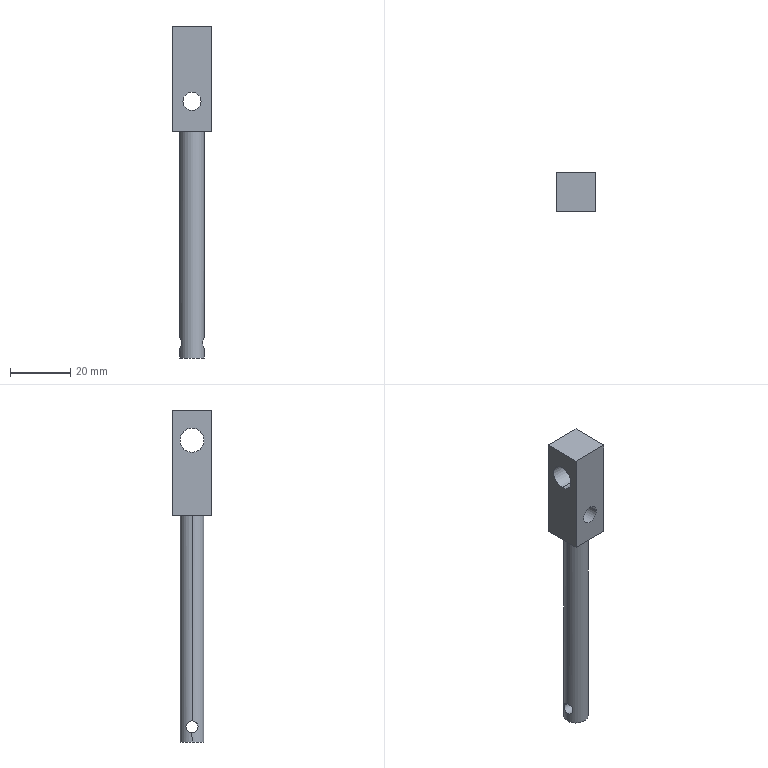Part | SolidWorks | features ICE 5, Extrusion 1 | 1 solid | 15 faces | box 13 x 13 x 110 mm | volume 8567 mm3 | cylinder 8 | plane 7 | commonest cylinder face diameters 8 x4 4 x2 6 x2
STEP:
#1=CARTESIAN_POINT('',(3.464,2.,-80.));
#2=VERTEX_POINT('',#1);
#3=CARTESIAN_POINT('',(4.,0.,-82.));
#4=VERTEX_POINT('',#3);
#5=CARTESIAN_POINT('',(3.464,2.,-80.));
#6=CARTESIAN_POINT('',(3.464,2.,-80.132));
#7=CARTESIAN_POINT('',(3.472,1.987,-80.266));
#8=CARTESIAN_POINT('',(3.501,1.934,-80.526));
#9=CARTESIAN_POINT('',(3.523,1.895,-80.652));
#10=CARTESIAN_POINT('',(3.602,1.744,-81.014));
#11=CARTESIAN_POINT('',(3.673,1.597,-81.231));
#12=CARTESIAN_POINT('',(3.776,1.324,-81.505));
#13=CARTESIAN_POINT('',(3.81,1.225,-81.586));
#14=CARTESIAN_POINT('',(3.872,1.011,-81.731));
#15=CARTESIAN_POINT('',(3.901,0.8943,-81.794));
#16=CARTESIAN_POINT('',(3.948,0.6536,-81.895));
#17=CARTESIAN_POINT('',(3.967,0.5287,-81.933));
#18=CARTESIAN_POINT('',(3.993,0.2692,-81.986));
#19=CARTESIAN_POINT('',(4.,0.1343,-82.));
#20=CARTESIAN_POINT('',(4.,0.,-82.));
#21=B_SPLINE_CURVE_WITH_KNOTS('',3,(#5,#6,#7,#8,#9,#10,#11,#12,#13,#14,#15,#16,#17,#18,#19,#20),.UNSPECIFIED.,.F.,.F.,(4,2,2,2,2,2,2,4),(0.00954,0.009936,0.01033,0.01113,0.01152,0.01192,0.01232,0.01271),.UNSPECIFIED.);
#22=EDGE_CURVE('',#2,#4,#21,.T.);
#23=ORIENTED_EDGE('',*,*,#22,.F.);
#24=CARTESIAN_POINT('',(-3.464,2.,-80.));
#25=VERTEX_POINT('',#24);
#26=CARTESIAN_POINT('',(293.5,2.,-80.));
#27=DIRECTION('',(-1.,0.,0.));
#28=VECTOR('',#27,1000.);
#29=LINE('',#26,#28);
#30=EDGE_CURVE('',#2,#25,#29,.T.);
#31=ORIENTED_EDGE('',*,*,#30,.T.);
#32=CARTESIAN_POINT('',(-4.,0.,-82.));
#33=VERTEX_POINT('',#32);
#34=CARTESIAN_POINT('',(-4.,0.,-82.));
#35=CARTESIAN_POINT('',(-4.,0.1332,-82.));
#36=CARTESIAN_POINT('',(-3.993,0.2678,-81.986));
#37=CARTESIAN_POINT('',(-3.967,0.5267,-81.934));
#38=CARTESIAN_POINT('',(-3.948,0.6539,-81.895));
#39=CARTESIAN_POINT('',(-3.9,0.8967,-81.793));
#40=CARTESIAN_POINT('',(-3.872,1.011,-81.731));
#41=CARTESIAN_POINT('',(-3.809,1.226,-81.586));
#42=CARTESIAN_POINT('',(-3.775,1.326,-81.502));
#43=CARTESIAN_POINT('',(-3.672,1.598,-81.23));
#44=CARTESIAN_POINT('',(-3.601,1.745,-81.011));
#45=CARTESIAN_POINT('',(-3.523,1.895,-80.652));
#46=CARTESIAN_POINT('',(-3.501,1.934,-80.525));
#47=CARTESIAN_POINT('',(-3.472,1.987,-80.264));
#48=CARTESIAN_POINT('',(-3.464,2.,-80.133));
#49=CARTESIAN_POINT('',(-3.464,2.,-80.));
#50=B_SPLINE_CURVE_WITH_KNOTS('',3,(#34,#35,#36,#37,#38,#39,#40,#41,#42,#43,#44,#45,#46,#47,#48,#49),.UNSPECIFIED.,.F.,.F.,(4,2,2,2,2,2,2,4),(0.003182,0.003579,0.003977,0.004374,0.004772,0.005566,0.005964,0.006361),.UNSPECIFIED.);
#51=EDGE_CURVE('',#33,#25,#50,.T.);
#52=ORIENTED_EDGE('',*,*,#51,.F.);
#53=CARTESIAN_POINT('',(-3.464,-2.,-80.));
#54=VERTEX_POINT('',#53);
#55=CARTESIAN_POINT('',(-3.464,-2.,-80.));
#56=CARTESIAN_POINT('',(-3.464,-2.,-80.135));
#57=CARTESIAN_POINT('',(-3.472,-1.987,-80.267));
#58=CARTESIAN_POINT('',(-3.501,-1.934,-80.525));
#59=CARTESIAN_POINT('',(-3.523,-1.895,-80.653));
#60=CARTESIAN_POINT('',(-3.602,-1.743,-81.015));
#61=CARTESIAN_POINT('',(-3.673,-1.596,-81.233));
#62=CARTESIAN_POINT('',(-3.81,-1.233,-81.596));
#63=CARTESIAN_POINT('',(-3.877,-1.014,-81.744));
#64=CARTESIAN_POINT('',(-3.948,-0.653,-81.895));
#65=CARTESIAN_POINT('',(-3.968,-0.5246,-81.935));
#66=CARTESIAN_POINT('',(-3.993,-0.2649,-81.987));
#67=CARTESIAN_POINT('',(-4.,-0.1333,-82.));
#68=CARTESIAN_POINT('',(-4.,0.,-82.));
#69=B_SPLINE_CURVE_WITH_KNOTS('',3,(#55,#56,#57,#58,#59,#60,#61,#62,#63,#64,#65,#66,#67,#68),.UNSPECIFIED.,.F.,.F.,(4,2,2,2,2,2,4),(0.,0.0003977,0.0007955,0.001591,0.002386,0.002784,0.003182),.UNSPECIFIED.);
#70=EDGE_CURVE('',#54,#33,#69,.T.);
#71=ORIENTED_EDGE('',*,*,#70,.F.);
#72=CARTESIAN_POINT('',(3.464,-2.,-80.));
#73=VERTEX_POINT('',#72);
#74=CARTESIAN_POINT('',(293.5,-2.,-80.));
#75=DIRECTION('',(-1.,0.,0.));
#76=VECTOR('',#75,1000.);
#77=LINE('',#74,#76);
#78=EDGE_CURVE('',#73,#54,#77,.T.);
#79=ORIENTED_EDGE('',*,*,#78,.F.);
#80=CARTESIAN_POINT('',(4.,0.,-82.));
#81=CARTESIAN_POINT('',(4.,-0.1347,-82.));
#82=CARTESIAN_POINT('',(3.993,-0.2667,-81.987));
#83=CARTESIAN_POINT('',(3.967,-0.5257,-81.934));
#84=CARTESIAN_POINT('',(3.948,-0.654,-81.895));
#85=CARTESIAN_POINT('',(3.877,-1.017,-81.742));
#86=CARTESIAN_POINT('',(3.809,-1.235,-81.594));
#87=CARTESIAN_POINT('',(3.672,-1.598,-81.23));
#88=CARTESIAN_POINT('',(3.601,-1.745,-81.012));
#89=CARTESIAN_POINT('',(3.523,-1.895,-80.652));
#90=CARTESIAN_POINT('',(3.501,-1.935,-80.524));
#91=CARTESIAN_POINT('',(3.472,-1.987,-80.265));
#92=CARTESIAN_POINT('',(3.464,-2.,-80.133));
#93=CARTESIAN_POINT('',(3.464,-2.,-80.));
#94=B_SPLINE_CURVE_WITH_KNOTS('',3,(#80,#81,#82,#83,#84,#85,#86,#87,#88,#89,#90,#91,#92,#93),.UNSPECIFIED.,.F.,.F.,(4,2,2,2,2,2,4),(0.,0.0003979,0.0007957,0.001591,0.002387,0.002785,0.003183),.UNSPECIFIED.);
#95=EDGE_CURVE('',#4,#73,#94,.T.);
#96=ORIENTED_EDGE('',*,*,#95,.F.);
#97=EDGE_LOOP('',(#23,#31,#52,#71,#79,#96));
#98=FACE_OUTER_BOUND('',#97,.T.);
#99=CARTESIAN_POINT('',(293.5,0.,-80.));
#100=DIRECTION('',(-1.,0.,0.));
#101=DIRECTION('',(0.,-1.,0.));
#102=AXIS2_PLACEMENT_3D('',#99,#100,#101);
#103=CYLINDRICAL_SURFACE('',#102,2.);
#104=ADVANCED_FACE('',(#98),#103,.F.);
#105=CARTESIAN_POINT('',(6.5,0.,11.));
#106=VERTEX_POINT('',#105);
#107=CARTESIAN_POINT('',(6.5,0.,19.));
#108=VERTEX_POINT('',#107);
#109=CARTESIAN_POINT('',(6.5,0.,15.));
#110=DIRECTION('',(-1.,0.,0.));
#111=DIRECTION('',(0.,0.,1.));
#112=AXIS2_PLACEMENT_3D('',#109,#110,#111);
#113=CIRCLE('',#112,4.);
#114=EDGE_CURVE('',#106,#108,#113,.T.);
#115=ORIENTED_EDGE('',*,*,#114,.F.);
#116=CARTESIAN_POINT('',(-6.5,0.,11.));
#117=VERTEX_POINT('',#116);
#118=CARTESIAN_POINT('',(30.5,0.,11.));
#119=DIRECTION('',(-1.,0.,0.));
#120=VECTOR('',#119,1000.);
#121=LINE('',#118,#120);
#122=EDGE_CURVE('',#106,#117,#121,.T.);
#123=ORIENTED_EDGE('',*,*,#122,.T.);
#124=CARTESIAN_POINT('',(-6.5,0.,19.));
#125=VERTEX_POINT('',#124);
#126=CARTESIAN_POINT('',(-6.5,0.,15.));
#127=DIRECTION('',(-1.,0.,0.));
#128=DIRECTION('',(0.,0.,1.));
#129=AXIS2_PLACEMENT_3D('',#126,#127,#128);
#130=CIRCLE('',#129,4.);
#131=EDGE_CURVE('',#117,#125,#130,.T.);
#132=ORIENTED_EDGE('',*,*,#131,.T.);
#133=CARTESIAN_POINT('',(30.5,0.,19.));
#134=DIRECTION('',(-1.,0.,0.));
#135=VECTOR('',#134,1000.);
#136=LINE('',#133,#135);
#137=EDGE_CURVE('',#108,#125,#136,.T.);
#138=ORIENTED_EDGE('',*,*,#137,.F.);
#139=EDGE_LOOP('',(#115,#123,#132,#138));
#140=FACE_OUTER_BOUND('',#139,.T.);
#141=CARTESIAN_POINT('',(30.5,0.,15.));
#142=DIRECTION('',(-1.,0.,0.));
#143=DIRECTION('',(0.,0.,1.));
#144=AXIS2_PLACEMENT_3D('',#141,#142,#143);
#145=CYLINDRICAL_SURFACE('',#144,4.);
#146=ADVANCED_FACE('',(#140),#145,.F.);
#147=CARTESIAN_POINT('',(-4.,0.,-85.));
#148=VERTEX_POINT('',#147);
#149=CARTESIAN_POINT('',(4.,0.,-85.));
#150=VERTEX_POINT('',#149);
#151=CARTESIAN_POINT('',(0.,0.,-85.));
#152=DIRECTION('',(0.,0.,-1.));
#153=DIRECTION('',(-1.,0.,0.));
#154=AXIS2_PLACEMENT_3D('',#151,#152,#153);
#155=CIRCLE('',#154,4.);
#156=EDGE_CURVE('',#148,#150,#155,.T.);
#157=ORIENTED_EDGE('',*,*,#156,.F.);
#158=CARTESIAN_POINT('',(-4.,0.,-85.));
#159=DIRECTION('',(0.,0.,1.));
#160=VECTOR('',#159,1000.);
#161=LINE('',#158,#160);
#162=EDGE_CURVE('',#148,#33,#161,.T.);
#163=ORIENTED_EDGE('',*,*,#162,.T.);
#164=ORIENTED_EDGE('',*,*,#51,.T.);
#165=CARTESIAN_POINT('',(-4.,0.,-78.));
#166=VERTEX_POINT('',#165);
#167=CARTESIAN_POINT('',(-3.464,2.,-80.));
#168=CARTESIAN_POINT('',(-3.464,2.,-79.868));
#169=CARTESIAN_POINT('',(-3.472,1.986,-79.733));
#170=CARTESIAN_POINT('',(-3.502,1.934,-79.473));
#171=CARTESIAN_POINT('',(-3.523,1.895,-79.348));
#172=CARTESIAN_POINT('',(-3.576,1.793,-79.105));
#173=CARTESIAN_POINT('',(-3.607,1.732,-78.991));
#174=CARTESIAN_POINT('',(-3.672,1.588,-78.777));
#175=CARTESIAN_POINT('',(-3.707,1.505,-78.676));
#176=CARTESIAN_POINT('',(-3.776,1.323,-78.494));
#177=CARTESIAN_POINT('',(-3.81,1.224,-78.413));
#178=CARTESIAN_POINT('',(-3.872,1.009,-78.268));
#179=CARTESIAN_POINT('',(-3.901,0.8925,-78.205));
#180=CARTESIAN_POINT('',(-3.972,0.5323,-78.055));
#181=CARTESIAN_POINT('',(-4.,0.2649,-78.));
#182=CARTESIAN_POINT('',(-4.,0.,-78.));
#183=B_SPLINE_CURVE_WITH_KNOTS('',3,(#167,#168,#169,#170,#171,#172,#173,#174,#175,#176,#177,#178,#179,#180,#181,#182),.UNSPECIFIED.,.F.,.F.,(4,2,2,2,2,2,2,4),(0.006361,0.006758,0.007155,0.007552,0.00795,0.008347,0.008744,0.009538),.UNSPECIFIED.);
#184=EDGE_CURVE('',#25,#166,#183,.T.);
#185=ORIENTED_EDGE('',*,*,#184,.T.);
#186=CARTESIAN_POINT('',(-4.,0.,-10.));
#187=VERTEX_POINT('',#186);
#188=CARTESIAN_POINT('',(-4.,0.,-85.));
#189=DIRECTION('',(0.,0.,1.));
#190=VECTOR('',#189,1000.);
#191=LINE('',#188,#190);
#192=EDGE_CURVE('',#166,#187,#191,.T.);
#193=ORIENTED_EDGE('',*,*,#192,.T.);
#194=CARTESIAN_POINT('',(4.,0.,-10.));
#195=VERTEX_POINT('',#194);
#196=CARTESIAN_POINT('',(0.,0.,-10.));
#197=DIRECTION('',(0.,0.,-1.));
#198=DIRECTION('',(-1.,0.,0.));
#199=AXIS2_PLACEMENT_3D('',#196,#197,#198);
#200=CIRCLE('',#199,4.);
#201=EDGE_CURVE('',#187,#195,#200,.T.);
#202=ORIENTED_EDGE('',*,*,#201,.T.);
#203=CARTESIAN_POINT('',(4.,0.,-78.));
#204=VERTEX_POINT('',#203);
#205=CARTESIAN_POINT('',(4.,0.,-85.));
#206=DIRECTION('',(0.,0.,1.));
#207=VECTOR('',#206,1000.);
#208=LINE('',#205,#207);
#209=EDGE_CURVE('',#204,#195,#208,.T.);
#210=ORIENTED_EDGE('',*,*,#209,.F.);
#211=CARTESIAN_POINT('',(4.,0.,-78.));
#212=CARTESIAN_POINT('',(4.,0.1327,-78.));
#213=CARTESIAN_POINT('',(3.993,0.2677,-78.014));
#214=CARTESIAN_POINT('',(3.967,0.527,-78.066));
#215=CARTESIAN_POINT('',(3.948,0.6528,-78.105));
#216=CARTESIAN_POINT('',(3.9,0.8965,-78.207));
#217=CARTESIAN_POINT('',(3.872,1.011,-78.269));
#218=CARTESIAN_POINT('',(3.809,1.225,-78.414));
#219=CARTESIAN_POINT('',(3.775,1.326,-78.497));
#220=CARTESIAN_POINT('',(3.706,1.508,-78.68));
#221=CARTESIAN_POINT('',(3.672,1.589,-78.779));
#222=CARTESIAN_POINT('',(3.606,1.733,-78.993));
#223=CARTESIAN_POINT('',(3.575,1.795,-79.109));
#224=CARTESIAN_POINT('',(3.523,1.895,-79.348));
#225=CARTESIAN_POINT('',(3.502,1.934,-79.473));
#226=CARTESIAN_POINT('',(3.472,1.987,-79.734));
#227=CARTESIAN_POINT('',(3.464,2.,-79.868));
#228=CARTESIAN_POINT('',(3.464,2.,-80.));
#229=B_SPLINE_CURVE_WITH_KNOTS('',3,(#211,#212,#213,#214,#215,#216,#217,#218,#219,#220,#221,#222,#223,#224,#225,#226,#227,#228),.UNSPECIFIED.,.F.,.F.,(4,2,2,2,2,2,2,2,4),(0.006362,0.006759,0.007156,0.007554,0.007951,0.008348,0.008745,0.009142,0.00954),.UNSPECIFIED.);
#230=EDGE_CURVE('',#204,#2,#229,.T.);
#231=ORIENTED_EDGE('',*,*,#230,.T.);
#232=ORIENTED_EDGE('',*,*,#22,.T.);
#233=CARTESIAN_POINT('',(4.,0.,-85.));
#234=DIRECTION('',(0.,0.,1.));
#235=VECTOR('',#234,1000.);
#236=LINE('',#233,#235);
#237=EDGE_CURVE('',#150,#4,#236,.T.);
#238=ORIENTED_EDGE('',*,*,#237,.F.);
#239=EDGE_LOOP('',(#157,#163,#164,#185,#193,#202,#210,#231,#232,#238));
#240=FACE_OUTER_BOUND('',#239,.T.);
#241=CARTESIAN_POINT('',(0.,0.,-85.));
#242=DIRECTION('',(0.,0.,1.));
#243=DIRECTION('',(1.,0.,0.));
#244=AXIS2_PLACEMENT_3D('',#241,#242,#243);
#245=CYLINDRICAL_SURFACE('',#244,4.);
#246=ADVANCED_FACE('',(#240),#245,.T.);
#247=CARTESIAN_POINT('',(3.,-6.5,0.));
#248=VERTEX_POINT('',#247);
#249=CARTESIAN_POINT('',(-3.,-6.5,0.));
#250=VERTEX_POINT('',#249);
#251=CARTESIAN_POINT('',(0.,-6.5,0.));
#252=DIRECTION('',(0.,1.,0.));
#253=DIRECTION('',(-1.,0.,0.));
#254=AXIS2_PLACEMENT_3D('',#251,#252,#253);
#255=CIRCLE('',#254,3.);
#256=EDGE_CURVE('',#248,#250,#255,.T.);
#257=ORIENTED_EDGE('',*,*,#256,.F.);
#258=CARTESIAN_POINT('',(3.,6.5,0.));
#259=VERTEX_POINT('',#258);
#260=CARTESIAN_POINT('',(3.,-13.5,0.));
#261=DIRECTION('',(0.,1.,0.));
#262=VECTOR('',#261,1000.);
#263=LINE('',#260,#262);
#264=EDGE_CURVE('',#248,#259,#263,.T.);
#265=ORIENTED_EDGE('',*,*,#264,.T.);
#266=CARTESIAN_POINT('',(-3.,6.5,0.));
#267=VERTEX_POINT('',#266);
#268=CARTESIAN_POINT('',(0.,6.5,0.));
#269=DIRECTION('',(0.,1.,0.));
#270=DIRECTION('',(-1.,0.,0.));
#271=AXIS2_PLACEMENT_3D('',#268,#269,#270);
#272=CIRCLE('',#271,3.);
#273=EDGE_CURVE('',#259,#267,#272,.T.);
#274=ORIENTED_EDGE('',*,*,#273,.T.);
#275=CARTESIAN_POINT('',(-3.,-13.5,0.));
#276=DIRECTION('',(0.,1.,0.));
#277=VECTOR('',#276,1000.);
#278=LINE('',#275,#277);
#279=EDGE_CURVE('',#250,#267,#278,.T.);
#280=ORIENTED_EDGE('',*,*,#279,.F.);
#281=EDGE_LOOP('',(#257,#265,#274,#280));
#282=FACE_OUTER_BOUND('',#281,.T.);
#283=CARTESIAN_POINT('',(0.,-13.5,0.));
#284=DIRECTION('',(0.,1.,0.));
#285=DIRECTION('',(-1.,0.,0.));
#286=AXIS2_PLACEMENT_3D('',#283,#284,#285);
#287=CYLINDRICAL_SURFACE('',#286,3.);
#288=ADVANCED_FACE('',(#282),#287,.F.);
#289=CARTESIAN_POINT('',(-6.5,0.,15.));
#290=DIRECTION('',(-1.,0.,0.));
#291=DIRECTION('',(0.,0.,1.));
#292=AXIS2_PLACEMENT_3D('',#289,#290,#291);
#293=CIRCLE('',#292,4.);
#294=EDGE_CURVE('',#125,#117,#293,.T.);
#295=ORIENTED_EDGE('',*,*,#294,.F.);
#296=ORIENTED_EDGE('',*,*,#131,.F.);
#297=EDGE_LOOP('',(#295,#296));
#298=FACE_BOUND('',#297,.T.);
#299=CARTESIAN_POINT('',(-6.5,6.5,-10.));
#300=VERTEX_POINT('',#299);
#301=CARTESIAN_POINT('',(-6.5,-6.5,-10.));
#302=VERTEX_POINT('',#301);
#303=CARTESIAN_POINT('',(-6.5,-6.5,-10.));
#304=DIRECTION('',(0.,-1.,0.));
#305=VECTOR('',#304,1000.);
#306=LINE('',#303,#305);
#307=EDGE_CURVE('',#300,#302,#306,.T.);
#308=ORIENTED_EDGE('',*,*,#307,.T.);
#309=CARTESIAN_POINT('',(-6.5,-6.5,25.));
#310=VERTEX_POINT('',#309);
#311=CARTESIAN_POINT('',(-6.5,-6.5,10.));
#312=DIRECTION('',(0.,0.,-1.));
#313=VECTOR('',#312,1000.);
#314=LINE('',#311,#313);
#315=EDGE_CURVE('',#310,#302,#314,.T.);
#316=ORIENTED_EDGE('',*,*,#315,.F.);
#317=CARTESIAN_POINT('',(-6.5,6.5,25.));
#318=VERTEX_POINT('',#317);
#319=CARTESIAN_POINT('',(-6.5,6.5,25.));
#320=DIRECTION('',(0.,-1.,0.));
#321=VECTOR('',#320,1000.);
#322=LINE('',#319,#321);
#323=EDGE_CURVE('',#318,#310,#322,.T.);
#324=ORIENTED_EDGE('',*,*,#323,.F.);
#325=CARTESIAN_POINT('',(-6.5,6.5,10.));
#326=DIRECTION('',(0.,0.,-1.));
#327=VECTOR('',#326,1000.);
#328=LINE('',#325,#327);
#329=EDGE_CURVE('',#318,#300,#328,.T.);
#330=ORIENTED_EDGE('',*,*,#329,.T.);
#331=EDGE_LOOP('',(#308,#316,#324,#330));
#332=FACE_OUTER_BOUND('',#331,.T.);
#333=CARTESIAN_POINT('',(-6.5,-6.5,10.));
#334=DIRECTION('',(1.,0.,0.));
#335=DIRECTION('',(0.,0.,-1.));
#336=AXIS2_PLACEMENT_3D('',#333,#334,#335);
#337=PLANE('',#336);
#338=ADVANCED_FACE('',(#298,#332),#337,.F.);
#339=CARTESIAN_POINT('',(0.,-6.5,0.));
#340=DIRECTION('',(0.,1.,0.));
#341=DIRECTION('',(-1.,0.,0.));
#342=AXIS2_PLACEMENT_3D('',#339,#340,#341);
#343=CIRCLE('',#342,3.);
#344=EDGE_CURVE('',#250,#248,#343,.T.);
#345=ORIENTED_EDGE('',*,*,#344,.T.);
#346=ORIENTED_EDGE('',*,*,#256,.T.);
#347=EDGE_LOOP('',(#345,#346));
#348=FACE_BOUND('',#347,.T.);
#349=CARTESIAN_POINT('',(6.5,-6.5,-10.));
#350=VERTEX_POINT('',#349);
#351=CARTESIAN_POINT('',(6.5,-6.5,-10.));
#352=DIRECTION('',(1.,0.,0.));
#353=VECTOR('',#352,1000.);
#354=LINE('',#351,#353);
#355=EDGE_CURVE('',#302,#350,#354,.T.);
#356=ORIENTED_EDGE('',*,*,#355,.T.);
#357=CARTESIAN_POINT('',(6.5,-6.5,25.));
#358=VERTEX_POINT('',#357);
#359=CARTESIAN_POINT('',(6.5,-6.5,10.));
#360=DIRECTION('',(0.,0.,-1.));
#361=VECTOR('',#360,1000.);
#362=LINE('',#359,#361);
#363=EDGE_CURVE('',#358,#350,#362,.T.);
#364=ORIENTED_EDGE('',*,*,#363,.F.);
#365=CARTESIAN_POINT('',(-6.5,-6.5,25.));
#366=DIRECTION('',(1.,0.,0.));
#367=VECTOR('',#366,1000.);
#368=LINE('',#365,#367);
#369=EDGE_CURVE('',#310,#358,#368,.T.);
#370=ORIENTED_EDGE('',*,*,#369,.F.);
#371=ORIENTED_EDGE('',*,*,#315,.T.);
#372=EDGE_LOOP('',(#356,#364,#370,#371));
#373=FACE_OUTER_BOUND('',#372,.T.);
#374=CARTESIAN_POINT('',(6.5,-6.5,10.));
#375=DIRECTION('',(0.,1.,0.));
#376=DIRECTION('',(-1.,0.,0.));
#377=AXIS2_PLACEMENT_3D('',#374,#375,#376);
#378=PLANE('',#377);
#379=ADVANCED_FACE('',(#348,#373),#378,.F.);
#380=CARTESIAN_POINT('',(6.5,0.,15.));
#381=DIRECTION('',(-1.,0.,0.));
#382=DIRECTION('',(0.,0.,1.));
#383=AXIS2_PLACEMENT_3D('',#380,#381,#382);
#384=CIRCLE('',#383,4.);
#385=EDGE_CURVE('',#108,#106,#384,.T.);
#386=ORIENTED_EDGE('',*,*,#385,.T.);
#387=ORIENTED_EDGE('',*,*,#114,.T.);
#388=EDGE_LOOP('',(#386,#387));
#389=FACE_BOUND('',#388,.T.);
#390=CARTESIAN_POINT('',(6.5,6.5,-10.));
#391=VERTEX_POINT('',#390);
#392=CARTESIAN_POINT('',(6.5,-6.5,-10.));
#393=DIRECTION('',(0.,1.,0.));
#394=VECTOR('',#393,1000.);
#395=LINE('',#392,#394);
#396=EDGE_CURVE('',#350,#391,#395,.T.);
#397=ORIENTED_EDGE('',*,*,#396,.T.);
#398=CARTESIAN_POINT('',(6.5,6.5,25.));
#399=VERTEX_POINT('',#398);
#400=CARTESIAN_POINT('',(6.5,6.5,10.));
#401=DIRECTION('',(0.,0.,-1.));
#402=VECTOR('',#401,1000.);
#403=LINE('',#400,#402);
#404=EDGE_CURVE('',#399,#391,#403,.T.);
#405=ORIENTED_EDGE('',*,*,#404,.F.);
#406=CARTESIAN_POINT('',(6.5,-6.5,25.));
#407=DIRECTION('',(0.,1.,0.));
#408=VECTOR('',#407,1000.);
#409=LINE('',#406,#408);
#410=EDGE_CURVE('',#358,#399,#409,.T.);
#411=ORIENTED_EDGE('',*,*,#410,.F.);
#412=ORIENTED_EDGE('',*,*,#363,.T.);
#413=EDGE_LOOP('',(#397,#405,#411,#412));
#414=FACE_OUTER_BOUND('',#413,.T.);
#415=CARTESIAN_POINT('',(6.5,-6.5,10.));
#416=DIRECTION('',(-1.,0.,0.));
#417=DIRECTION('',(0.,0.,1.));
#418=AXIS2_PLACEMENT_3D('',#415,#416,#417);
#419=PLANE('',#418);
#420=ADVANCED_FACE('',(#389,#414),#419,.F.);
#421=CARTESIAN_POINT('',(0.,6.5,0.));
#422=DIRECTION('',(0.,1.,0.));
#423=DIRECTION('',(-1.,0.,0.));
#424=AXIS2_PLACEMENT_3D('',#421,#422,#423);
#425=CIRCLE('',#424,3.);
#426=EDGE_CURVE('',#267,#259,#425,.T.);
#427=ORIENTED_EDGE('',*,*,#426,.F.);
#428=ORIENTED_EDGE('',*,*,#273,.F.);
#429=EDGE_LOOP('',(#427,#428));
#430=FACE_BOUND('',#429,.T.);
#431=CARTESIAN_POINT('',(6.5,6.5,-10.));
#432=DIRECTION('',(-1.,0.,0.));
#433=VECTOR('',#432,1000.);
#434=LINE('',#431,#433);
#435=EDGE_CURVE('',#391,#300,#434,.T.);
#436=ORIENTED_EDGE('',*,*,#435,.T.);
#437=ORIENTED_EDGE('',*,*,#329,.F.);
#438=CARTESIAN_POINT('',(6.5,6.5,25.));
#439=DIRECTION('',(-1.,0.,0.));
#440=VECTOR('',#439,1000.);
#441=LINE('',#438,#440);
#442=EDGE_CURVE('',#399,#318,#441,.T.);
#443=ORIENTED_EDGE('',*,*,#442,.F.);
#444=ORIENTED_EDGE('',*,*,#404,.T.);
#445=EDGE_LOOP('',(#436,#437,#443,#444));
#446=FACE_OUTER_BOUND('',#445,.T.);
#447=CARTESIAN_POINT('',(6.5,6.5,10.));
#448=DIRECTION('',(0.,-1.,0.));
#449=DIRECTION('',(1.,0.,0.));
#450=AXIS2_PLACEMENT_3D('',#447,#448,#449);
#451=PLANE('',#450);
#452=ADVANCED_FACE('',(#430,#446),#451,.F.);
#453=CARTESIAN_POINT('',(0.,0.,-10.));
#454=DIRECTION('',(0.,0.,-1.));
#455=DIRECTION('',(-1.,0.,0.));
#456=AXIS2_PLACEMENT_3D('',#453,#454,#455);
#457=CIRCLE('',#456,4.);
#458=EDGE_CURVE('',#195,#187,#457,.T.);
#459=ORIENTED_EDGE('',*,*,#458,.F.);
#460=ORIENTED_EDGE('',*,*,#201,.F.);
#461=EDGE_LOOP('',(#459,#460));
#462=FACE_BOUND('',#461,.T.);
#463=ORIENTED_EDGE('',*,*,#307,.F.);
#464=ORIENTED_EDGE('',*,*,#435,.F.);
#465=ORIENTED_EDGE('',*,*,#396,.F.);
#466=ORIENTED_EDGE('',*,*,#355,.F.);
#467=EDGE_LOOP('',(#463,#464,#465,#466));
#468=FACE_OUTER_BOUND('',#467,.T.);
#469=CARTESIAN_POINT('',(0.,0.,-10.));
#470=DIRECTION('',(0.,0.,1.));
#471=DIRECTION('',(1.,0.,0.));
#472=AXIS2_PLACEMENT_3D('',#469,#470,#471);
#473=PLANE('',#472);
#474=ADVANCED_FACE('',(#462,#468),#473,.F.);
#475=ORIENTED_EDGE('',*,*,#264,.F.);
#476=ORIENTED_EDGE('',*,*,#344,.F.);
#477=ORIENTED_EDGE('',*,*,#279,.T.);
#478=ORIENTED_EDGE('',*,*,#426,.T.);
#479=EDGE_LOOP('',(#475,#476,#477,#478));
#480=FACE_OUTER_BOUND('',#479,.T.);
#481=CARTESIAN_POINT('',(0.,-13.5,0.));
#482=DIRECTION('',(0.,1.,0.));
#483=DIRECTION('',(-1.,0.,0.));
#484=AXIS2_PLACEMENT_3D('',#481,#482,#483);
#485=CYLINDRICAL_SURFACE('',#484,3.);
#486=ADVANCED_FACE('',(#480),#485,.F.);
#487=ORIENTED_EDGE('',*,*,#162,.F.);
#488=CARTESIAN_POINT('',(0.,0.,-85.));
#489=DIRECTION('',(0.,0.,-1.));
#490=DIRECTION('',(-1.,0.,0.));
#491=AXIS2_PLACEMENT_3D('',#488,#489,#490);
#492=CIRCLE('',#491,4.);
#493=EDGE_CURVE('',#150,#148,#492,.T.);
#494=ORIENTED_EDGE('',*,*,#493,.F.);
#495=ORIENTED_EDGE('',*,*,#237,.T.);
#496=ORIENTED_EDGE('',*,*,#95,.T.);
#497=CARTESIAN_POINT('',(3.464,-2.,-80.));
#498=CARTESIAN_POINT('',(3.464,-2.,-79.867));
#499=CARTESIAN_POINT('',(3.472,-1.986,-79.732));
#500=CARTESIAN_POINT('',(3.502,-1.934,-79.474));
#501=CARTESIAN_POINT('',(3.523,-1.895,-79.347));
#502=CARTESIAN_POINT('',(3.576,-1.793,-79.105));
#503=CARTESIAN_POINT('',(3.607,-1.732,-78.991));
#504=CARTESIAN_POINT('',(3.672,-1.587,-78.776));
#505=CARTESIAN_POINT('',(3.708,-1.504,-78.676));
#506=CARTESIAN_POINT('',(3.81,-1.232,-78.404));
#507=CARTESIAN_POINT('',(3.877,-1.013,-78.256));
#508=CARTESIAN_POINT('',(3.948,-0.6526,-78.105));
#509=CARTESIAN_POINT('',(3.967,-0.5257,-78.066));
#510=CARTESIAN_POINT('',(3.993,-0.2644,-78.013));
#511=CARTESIAN_POINT('',(4.,-0.1327,-78.));
#512=CARTESIAN_POINT('',(4.,0.,-78.));
#513=B_SPLINE_CURVE_WITH_KNOTS('',3,(#497,#498,#499,#500,#501,#502,#503,#504,#505,#506,#507,#508,#509,#510,#511,#512),.UNSPECIFIED.,.F.,.F.,(4,2,2,2,2,2,2,4),(0.003183,0.00358,0.003978,0.004375,0.004772,0.005567,0.005965,0.006362),.UNSPECIFIED.);
#514=EDGE_CURVE('',#73,#204,#513,.T.);
#515=ORIENTED_EDGE('',*,*,#514,.T.);
#516=ORIENTED_EDGE('',*,*,#209,.T.);
#517=ORIENTED_EDGE('',*,*,#458,.T.);
#518=ORIENTED_EDGE('',*,*,#192,.F.);
#519=CARTESIAN_POINT('',(-4.,0.,-78.));
#520=CARTESIAN_POINT('',(-4.,-0.1323,-78.));
#521=CARTESIAN_POINT('',(-3.993,-0.2666,-78.013));
#522=CARTESIAN_POINT('',(-3.967,-0.5268,-78.066));
#523=CARTESIAN_POINT('',(-3.948,-0.6523,-78.105));
#524=CARTESIAN_POINT('',(-3.877,-1.016,-78.257));
#525=CARTESIAN_POINT('',(-3.81,-1.234,-78.405));
#526=CARTESIAN_POINT('',(-3.707,-1.507,-78.679));
#527=CARTESIAN_POINT('',(-3.672,-1.588,-78.778));
#528=CARTESIAN_POINT('',(-3.607,-1.732,-78.991));
#529=CARTESIAN_POINT('',(-3.575,-1.794,-79.107));
#530=CARTESIAN_POINT('',(-3.523,-1.895,-79.347));
#531=CARTESIAN_POINT('',(-3.502,-1.933,-79.472));
#532=CARTESIAN_POINT('',(-3.472,-1.986,-79.731));
#533=CARTESIAN_POINT('',(-3.464,-2.,-79.866));
#534=CARTESIAN_POINT('',(-3.464,-2.,-80.));
#535=B_SPLINE_CURVE_WITH_KNOTS('',3,(#519,#520,#521,#522,#523,#524,#525,#526,#527,#528,#529,#530,#531,#532,#533,#534),.UNSPECIFIED.,.F.,.F.,(4,2,2,2,2,2,2,4),(0.009538,0.009935,0.01033,0.01112,0.01152,0.01192,0.01231,0.01271),.UNSPECIFIED.);
#536=EDGE_CURVE('',#166,#54,#535,.T.);
#537=ORIENTED_EDGE('',*,*,#536,.T.);
#538=ORIENTED_EDGE('',*,*,#70,.T.);
#539=EDGE_LOOP('',(#487,#494,#495,#496,#515,#516,#517,#518,#537,#538));
#540=FACE_OUTER_BOUND('',#539,.T.);
#541=CARTESIAN_POINT('',(0.,0.,-85.));
#542=DIRECTION('',(0.,0.,1.));
#543=DIRECTION('',(1.,0.,0.));
#544=AXIS2_PLACEMENT_3D('',#541,#542,#543);
#545=CYLINDRICAL_SURFACE('',#544,4.);
#546=ADVANCED_FACE('',(#540),#545,.T.);
#547=ORIENTED_EDGE('',*,*,#493,.T.);
#548=ORIENTED_EDGE('',*,*,#156,.T.);
#549=EDGE_LOOP('',(#547,#548));
#550=FACE_OUTER_BOUND('',#549,.T.);
#551=CARTESIAN_POINT('',(0.,0.,-85.));
#552=DIRECTION('',(0.,0.,-1.));
#553=DIRECTION('',(-1.,0.,0.));
#554=AXIS2_PLACEMENT_3D('',#551,#552,#553);
#555=PLANE('',#554);
#556=ADVANCED_FACE('',(#550),#555,.T.);
#557=ORIENTED_EDGE('',*,*,#442,.T.);
#558=ORIENTED_EDGE('',*,*,#323,.T.);
#559=ORIENTED_EDGE('',*,*,#369,.T.);
#560=ORIENTED_EDGE('',*,*,#410,.T.);
#561=EDGE_LOOP('',(#557,#558,#559,#560));
#562=FACE_OUTER_BOUND('',#561,.T.);
#563=CARTESIAN_POINT('',(0.,0.,25.));
#564=DIRECTION('',(0.,0.,1.));
#565=DIRECTION('',(1.,0.,0.));
#566=AXIS2_PLACEMENT_3D('',#563,#564,#565);
#567=PLANE('',#566);
#568=ADVANCED_FACE('',(#562),#567,.T.);
#569=ORIENTED_EDGE('',*,*,#122,.F.);
#570=ORIENTED_EDGE('',*,*,#385,.F.);
#571=ORIENTED_EDGE('',*,*,#137,.T.);
#572=ORIENTED_EDGE('',*,*,#294,.T.);
#573=EDGE_LOOP('',(#569,#570,#571,#572));
#574=FACE_OUTER_BOUND('',#573,.T.);
#575=CARTESIAN_POINT('',(30.5,0.,15.));
#576=DIRECTION('',(-1.,0.,0.));
#577=DIRECTION('',(0.,0.,1.));
#578=AXIS2_PLACEMENT_3D('',#575,#576,#577);
#579=CYLINDRICAL_SURFACE('',#578,4.);
#580=ADVANCED_FACE('',(#574),#579,.F.);
#581=ORIENTED_EDGE('',*,*,#30,.F.);
#582=ORIENTED_EDGE('',*,*,#230,.F.);
#583=ORIENTED_EDGE('',*,*,#514,.F.);
#584=ORIENTED_EDGE('',*,*,#78,.T.);
#585=ORIENTED_EDGE('',*,*,#536,.F.);
#586=ORIENTED_EDGE('',*,*,#184,.F.);
#587=EDGE_LOOP('',(#581,#582,#583,#584,#585,#586));
#588=FACE_OUTER_BOUND('',#587,.T.);
#589=CARTESIAN_POINT('',(293.5,0.,-80.));
#590=DIRECTION('',(-1.,0.,0.));
#591=DIRECTION('',(0.,-1.,0.));
#592=AXIS2_PLACEMENT_3D('',#589,#590,#591);
#593=CYLINDRICAL_SURFACE('',#592,2.);
#594=ADVANCED_FACE('',(#588),#593,.F.);
#595=CLOSED_SHELL('',(#104,#146,#246,#288,#338,#379,#420,#452,#474,#486,#546,#556,#568,#580,#594));
#596=MANIFOLD_SOLID_BREP('',#595);
#597=CARTESIAN_POINT('',(0.,0.,0.));
#598=DIRECTION('',(0.,0.,1.));
#599=DIRECTION('',(1.,0.,0.));
#600=AXIS2_PLACEMENT_3D('',#597,#598,#599);
#601=(LENGTH_UNIT()NAMED_UNIT(*)SI_UNIT(.MILLI.,.METRE.));
#602=UNCERTAINTY_MEASURE_WITH_UNIT(LENGTH_MEASURE(0.00001),#601,'','');
#603=(NAMED_UNIT(*)PLANE_ANGLE_UNIT()SI_UNIT($,.RADIAN.));
#604=(NAMED_UNIT(*)SI_UNIT($,.STERADIAN.)SOLID_ANGLE_UNIT());
#605=(GEOMETRIC_REPRESENTATION_CONTEXT(3)GLOBAL_UNCERTAINTY_ASSIGNED_CONTEXT((#602))GLOBAL_UNIT_ASSIGNED_CONTEXT((#601,#603,#604))REPRESENTATION_CONTEXT('',''));
#606=ADVANCED_BREP_SHAPE_REPRESENTATION('',(#596,#600),#605);